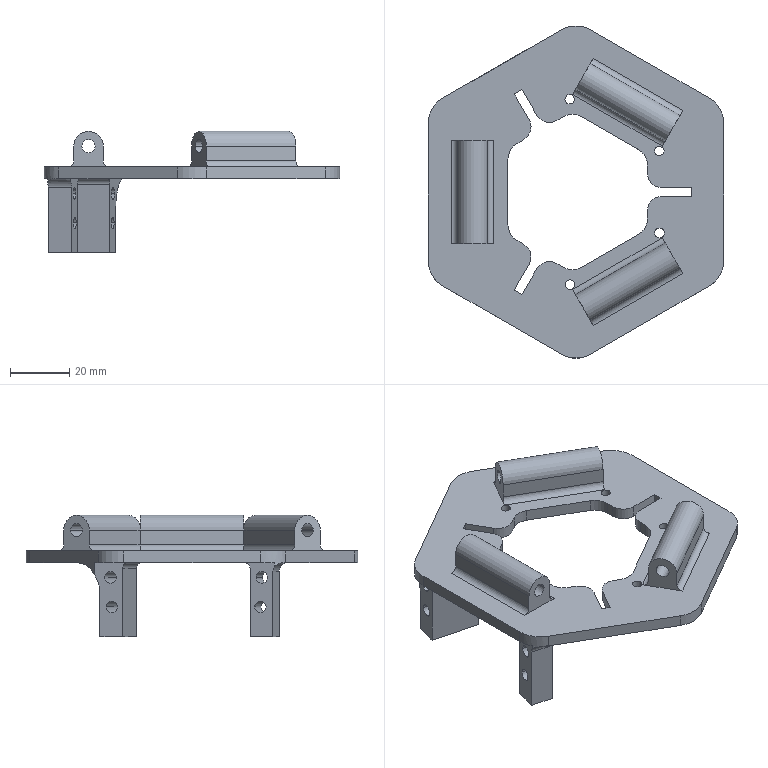Part | SolidWorks | features ICE 8, Fillet 7, Cut 3, CirPattern 2, Extrusion 1, RefAxis 1 | 1 solid | 108 faces | box 100 x 112.376 x 41 mm | volume 40931 mm3 | cylinder 58 | plane 50 | commonest cylinder face diameters 4 x16 10 x10 3.2 x8 20 x7 4.5 x6 12 x6